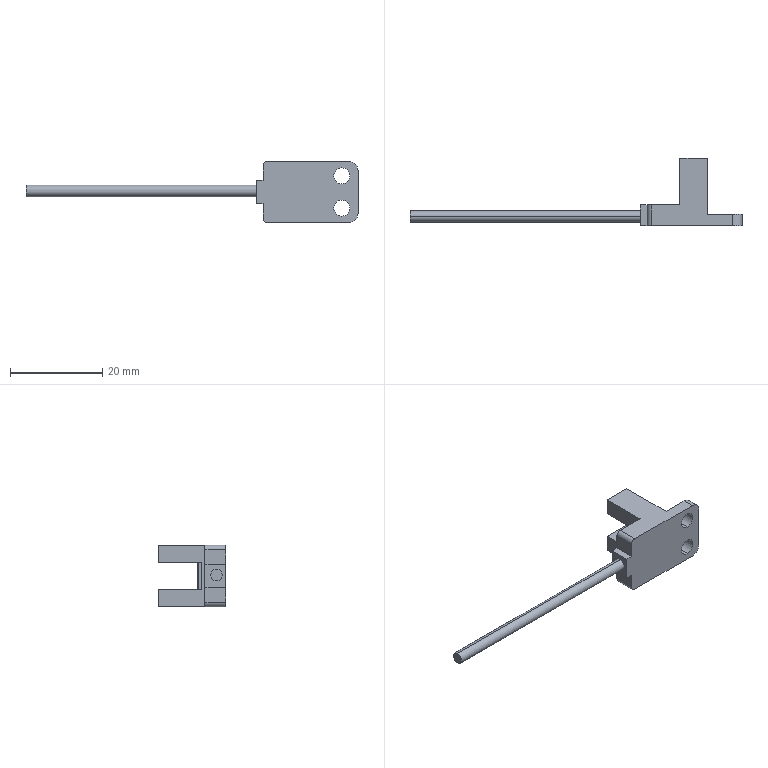Part | NX | features BREP 1 | 1 solid | 61 faces | box 72.1 x 14.6 x 13.4 mm | volume 1769 mm3 | plane 51 | cylinder 10 | commonest cylinder face diameters 3.5 x4 2 x2 2.5 x2 4 x2